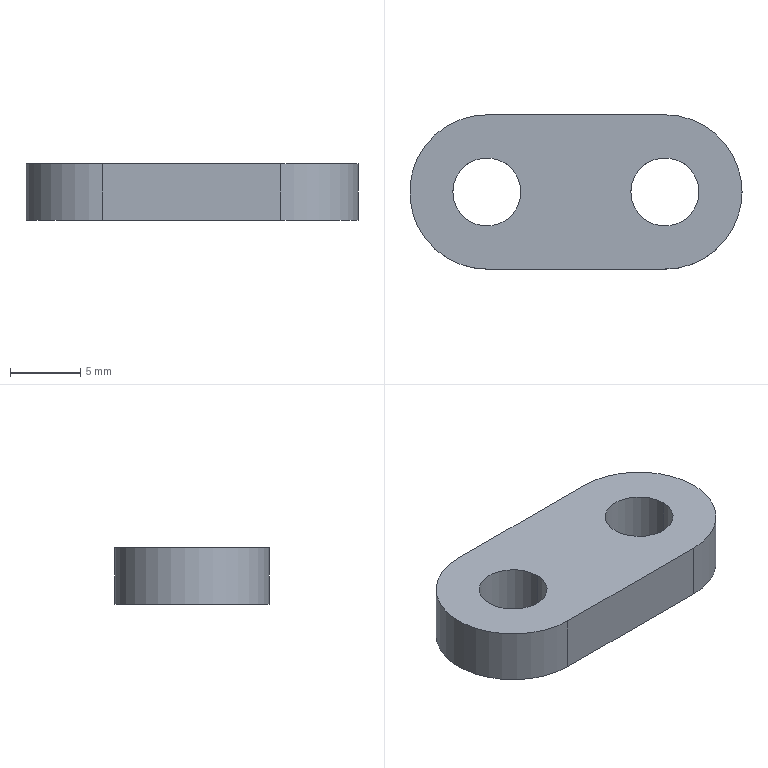Part | STEP file | 11-LINK_MC01-S311 | 1 solid | 11 faces | box 23.697 x 11 x 4 mm | volume 791.004 mm3 | cylinder 7 | plane 4 | commonest cylinder face diameters 4.85 x4 11 x3
STEP:
#1=CARTESIAN_POINT('',(-2.425,0.,-4.));
#2=VERTEX_POINT('',#1);
#3=CARTESIAN_POINT('',(2.425,0.,-4.));
#4=VERTEX_POINT('',#3);
#5=CARTESIAN_POINT('',(0.,0.,-4.));
#6=DIRECTION('',(0.,0.,1.));
#7=DIRECTION('',(1.,0.,0.));
#8=AXIS2_PLACEMENT_3D('',#5,#6,#7);
#9=CIRCLE('',#8,2.425);
#10=EDGE_CURVE('',#2,#4,#9,.T.);
#11=ORIENTED_EDGE('',*,*,#10,.F.);
#12=CARTESIAN_POINT('',(-2.425,0.,0.));
#13=VERTEX_POINT('',#12);
#14=CARTESIAN_POINT('',(-2.425,0.,0.));
#15=DIRECTION('',(0.,0.,1.));
#16=VECTOR('',#15,1000.);
#17=LINE('',#14,#16);
#18=EDGE_CURVE('',#2,#13,#17,.T.);
#19=ORIENTED_EDGE('',*,*,#18,.T.);
#20=CARTESIAN_POINT('',(2.425,0.,0.));
#21=VERTEX_POINT('',#20);
#22=CARTESIAN_POINT('',(0.,0.,0.));
#23=DIRECTION('',(0.,0.,1.));
#24=DIRECTION('',(1.,0.,0.));
#25=AXIS2_PLACEMENT_3D('',#22,#23,#24);
#26=CIRCLE('',#25,2.425);
#27=EDGE_CURVE('',#13,#21,#26,.T.);
#28=ORIENTED_EDGE('',*,*,#27,.T.);
#29=CARTESIAN_POINT('',(2.425,0.,0.));
#30=DIRECTION('',(0.,0.,1.));
#31=VECTOR('',#30,1000.);
#32=LINE('',#29,#31);
#33=EDGE_CURVE('',#4,#21,#32,.T.);
#34=ORIENTED_EDGE('',*,*,#33,.F.);
#35=EDGE_LOOP('',(#11,#19,#28,#34));
#36=FACE_OUTER_BOUND('',#35,.T.);
#37=CARTESIAN_POINT('',(0.,0.,0.));
#38=DIRECTION('',(0.,0.,1.));
#39=DIRECTION('',(1.,0.,0.));
#40=AXIS2_PLACEMENT_3D('',#37,#38,#39);
#41=CYLINDRICAL_SURFACE('',#40,2.425);
#42=ADVANCED_FACE('',(#36),#41,.F.);
#43=CARTESIAN_POINT('',(10.272,0.,-4.));
#44=VERTEX_POINT('',#43);
#45=CARTESIAN_POINT('',(15.122,0.,-4.));
#46=VERTEX_POINT('',#45);
#47=CARTESIAN_POINT('',(12.697,0.,-4.));
#48=DIRECTION('',(0.,0.,1.));
#49=DIRECTION('',(1.,0.,0.));
#50=AXIS2_PLACEMENT_3D('',#47,#48,#49);
#51=CIRCLE('',#50,2.425);
#52=EDGE_CURVE('',#44,#46,#51,.T.);
#53=ORIENTED_EDGE('',*,*,#52,.F.);
#54=CARTESIAN_POINT('',(10.272,0.,0.));
#55=VERTEX_POINT('',#54);
#56=CARTESIAN_POINT('',(10.272,0.,0.));
#57=DIRECTION('',(0.,0.,1.));
#58=VECTOR('',#57,1000.);
#59=LINE('',#56,#58);
#60=EDGE_CURVE('',#44,#55,#59,.T.);
#61=ORIENTED_EDGE('',*,*,#60,.T.);
#62=CARTESIAN_POINT('',(15.122,0.,0.));
#63=VERTEX_POINT('',#62);
#64=CARTESIAN_POINT('',(12.697,0.,0.));
#65=DIRECTION('',(0.,0.,1.));
#66=DIRECTION('',(1.,0.,0.));
#67=AXIS2_PLACEMENT_3D('',#64,#65,#66);
#68=CIRCLE('',#67,2.425);
#69=EDGE_CURVE('',#55,#63,#68,.T.);
#70=ORIENTED_EDGE('',*,*,#69,.T.);
#71=CARTESIAN_POINT('',(15.122,0.,0.));
#72=DIRECTION('',(0.,0.,1.));
#73=VECTOR('',#72,1000.);
#74=LINE('',#71,#73);
#75=EDGE_CURVE('',#46,#63,#74,.T.);
#76=ORIENTED_EDGE('',*,*,#75,.F.);
#77=EDGE_LOOP('',(#53,#61,#70,#76));
#78=FACE_OUTER_BOUND('',#77,.T.);
#79=CARTESIAN_POINT('',(12.697,0.,0.));
#80=DIRECTION('',(0.,0.,1.));
#81=DIRECTION('',(1.,0.,0.));
#82=AXIS2_PLACEMENT_3D('',#79,#80,#81);
#83=CYLINDRICAL_SURFACE('',#82,2.425);
#84=ADVANCED_FACE('',(#78),#83,.F.);
#85=CARTESIAN_POINT('',(12.697,-5.5,-4.));
#86=VERTEX_POINT('',#85);
#87=CARTESIAN_POINT('',(18.197,0.,-4.));
#88=VERTEX_POINT('',#87);
#89=CARTESIAN_POINT('',(12.697,0.,-4.));
#90=DIRECTION('',(0.,0.,1.));
#91=DIRECTION('',(1.,0.,0.));
#92=AXIS2_PLACEMENT_3D('',#89,#90,#91);
#93=CIRCLE('',#92,5.5);
#94=EDGE_CURVE('',#86,#88,#93,.T.);
#95=ORIENTED_EDGE('',*,*,#94,.T.);
#96=CARTESIAN_POINT('',(18.197,0.,0.));
#97=VERTEX_POINT('',#96);
#98=CARTESIAN_POINT('',(18.197,0.,-4.));
#99=DIRECTION('',(0.,0.,1.));
#100=VECTOR('',#99,1000.);
#101=LINE('',#98,#100);
#102=EDGE_CURVE('',#88,#97,#101,.T.);
#103=ORIENTED_EDGE('',*,*,#102,.T.);
#104=CARTESIAN_POINT('',(12.697,-5.5,0.));
#105=VERTEX_POINT('',#104);
#106=CARTESIAN_POINT('',(12.697,0.,0.));
#107=DIRECTION('',(0.,0.,1.));
#108=DIRECTION('',(1.,0.,0.));
#109=AXIS2_PLACEMENT_3D('',#106,#107,#108);
#110=CIRCLE('',#109,5.5);
#111=EDGE_CURVE('',#105,#97,#110,.T.);
#112=ORIENTED_EDGE('',*,*,#111,.F.);
#113=CARTESIAN_POINT('',(12.697,-5.5,-4.));
#114=DIRECTION('',(0.,0.,1.));
#115=VECTOR('',#114,1000.);
#116=LINE('',#113,#115);
#117=EDGE_CURVE('',#86,#105,#116,.T.);
#118=ORIENTED_EDGE('',*,*,#117,.F.);
#119=EDGE_LOOP('',(#95,#103,#112,#118));
#120=FACE_OUTER_BOUND('',#119,.T.);
#121=CARTESIAN_POINT('',(12.697,0.,-4.));
#122=DIRECTION('',(0.,0.,1.));
#123=DIRECTION('',(1.,0.,0.));
#124=AXIS2_PLACEMENT_3D('',#121,#122,#123);
#125=CYLINDRICAL_SURFACE('',#124,5.5);
#126=ADVANCED_FACE('',(#120),#125,.T.);
#127=CARTESIAN_POINT('',(0.,5.5,0.));
#128=VERTEX_POINT('',#127);
#129=CARTESIAN_POINT('',(0.,-5.5,0.));
#130=VERTEX_POINT('',#129);
#131=CARTESIAN_POINT('',(0.,0.,0.));
#132=DIRECTION('',(0.,0.,1.));
#133=DIRECTION('',(1.,0.,0.));
#134=AXIS2_PLACEMENT_3D('',#131,#132,#133);
#135=CIRCLE('',#134,5.5);
#136=EDGE_CURVE('',#128,#130,#135,.T.);
#137=ORIENTED_EDGE('',*,*,#136,.F.);
#138=CARTESIAN_POINT('',(0.,5.5,-4.));
#139=VERTEX_POINT('',#138);
#140=CARTESIAN_POINT('',(0.,5.5,-4.));
#141=DIRECTION('',(0.,0.,1.));
#142=VECTOR('',#141,1000.);
#143=LINE('',#140,#142);
#144=EDGE_CURVE('',#139,#128,#143,.T.);
#145=ORIENTED_EDGE('',*,*,#144,.F.);
#146=CARTESIAN_POINT('',(0.,-5.5,-4.));
#147=VERTEX_POINT('',#146);
#148=CARTESIAN_POINT('',(0.,0.,-4.));
#149=DIRECTION('',(0.,0.,1.));
#150=DIRECTION('',(1.,0.,0.));
#151=AXIS2_PLACEMENT_3D('',#148,#149,#150);
#152=CIRCLE('',#151,5.5);
#153=EDGE_CURVE('',#139,#147,#152,.T.);
#154=ORIENTED_EDGE('',*,*,#153,.T.);
#155=CARTESIAN_POINT('',(0.,-5.5,-4.));
#156=DIRECTION('',(0.,0.,1.));
#157=VECTOR('',#156,1000.);
#158=LINE('',#155,#157);
#159=EDGE_CURVE('',#147,#130,#158,.T.);
#160=ORIENTED_EDGE('',*,*,#159,.T.);
#161=EDGE_LOOP('',(#137,#145,#154,#160));
#162=FACE_OUTER_BOUND('',#161,.T.);
#163=CARTESIAN_POINT('',(0.,0.,-4.));
#164=DIRECTION('',(0.,0.,1.));
#165=DIRECTION('',(1.,0.,0.));
#166=AXIS2_PLACEMENT_3D('',#163,#164,#165);
#167=CYLINDRICAL_SURFACE('',#166,5.5);
#168=ADVANCED_FACE('',(#162),#167,.T.);
#169=CARTESIAN_POINT('',(12.697,5.5,0.));
#170=VERTEX_POINT('',#169);
#171=CARTESIAN_POINT('',(0.,5.5,0.));
#172=DIRECTION('',(-1.,0.,0.));
#173=VECTOR('',#172,1000.);
#174=LINE('',#171,#173);
#175=EDGE_CURVE('',#170,#128,#174,.T.);
#176=ORIENTED_EDGE('',*,*,#175,.F.);
#177=CARTESIAN_POINT('',(12.697,5.5,-4.));
#178=VERTEX_POINT('',#177);
#179=CARTESIAN_POINT('',(12.697,5.5,-4.));
#180=DIRECTION('',(0.,0.,1.));
#181=VECTOR('',#180,1000.);
#182=LINE('',#179,#181);
#183=EDGE_CURVE('',#178,#170,#182,.T.);
#184=ORIENTED_EDGE('',*,*,#183,.F.);
#185=CARTESIAN_POINT('',(0.,5.5,-4.));
#186=DIRECTION('',(-1.,0.,0.));
#187=VECTOR('',#186,1000.);
#188=LINE('',#185,#187);
#189=EDGE_CURVE('',#178,#139,#188,.T.);
#190=ORIENTED_EDGE('',*,*,#189,.T.);
#191=ORIENTED_EDGE('',*,*,#144,.T.);
#192=EDGE_LOOP('',(#176,#184,#190,#191));
#193=FACE_OUTER_BOUND('',#192,.T.);
#194=CARTESIAN_POINT('',(0.,5.5,-4.));
#195=DIRECTION('',(0.,1.,0.));
#196=DIRECTION('',(0.,0.,1.));
#197=AXIS2_PLACEMENT_3D('',#194,#195,#196);
#198=PLANE('',#197);
#199=ADVANCED_FACE('',(#193),#198,.T.);
#200=ORIENTED_EDGE('',*,*,#102,.F.);
#201=CARTESIAN_POINT('',(12.697,0.,-4.));
#202=DIRECTION('',(0.,0.,1.));
#203=DIRECTION('',(1.,0.,0.));
#204=AXIS2_PLACEMENT_3D('',#201,#202,#203);
#205=CIRCLE('',#204,5.5);
#206=EDGE_CURVE('',#88,#178,#205,.T.);
#207=ORIENTED_EDGE('',*,*,#206,.T.);
#208=ORIENTED_EDGE('',*,*,#183,.T.);
#209=CARTESIAN_POINT('',(12.697,0.,0.));
#210=DIRECTION('',(0.,0.,1.));
#211=DIRECTION('',(1.,0.,0.));
#212=AXIS2_PLACEMENT_3D('',#209,#210,#211);
#213=CIRCLE('',#212,5.5);
#214=EDGE_CURVE('',#97,#170,#213,.T.);
#215=ORIENTED_EDGE('',*,*,#214,.F.);
#216=EDGE_LOOP('',(#200,#207,#208,#215));
#217=FACE_OUTER_BOUND('',#216,.T.);
#218=CARTESIAN_POINT('',(12.697,0.,-4.));
#219=DIRECTION('',(0.,0.,1.));
#220=DIRECTION('',(1.,0.,0.));
#221=AXIS2_PLACEMENT_3D('',#218,#219,#220);
#222=CYLINDRICAL_SURFACE('',#221,5.5);
#223=ADVANCED_FACE('',(#217),#222,.T.);
#224=CARTESIAN_POINT('',(0.,-5.5,0.));
#225=DIRECTION('',(1.,0.,0.));
#226=VECTOR('',#225,1000.);
#227=LINE('',#224,#226);
#228=EDGE_CURVE('',#130,#105,#227,.T.);
#229=ORIENTED_EDGE('',*,*,#228,.F.);
#230=ORIENTED_EDGE('',*,*,#159,.F.);
#231=CARTESIAN_POINT('',(0.,-5.5,-4.));
#232=DIRECTION('',(1.,0.,0.));
#233=VECTOR('',#232,1000.);
#234=LINE('',#231,#233);
#235=EDGE_CURVE('',#147,#86,#234,.T.);
#236=ORIENTED_EDGE('',*,*,#235,.T.);
#237=ORIENTED_EDGE('',*,*,#117,.T.);
#238=EDGE_LOOP('',(#229,#230,#236,#237));
#239=FACE_OUTER_BOUND('',#238,.T.);
#240=CARTESIAN_POINT('',(0.,-5.5,-4.));
#241=DIRECTION('',(0.,-1.,0.));
#242=DIRECTION('',(0.,0.,-1.));
#243=AXIS2_PLACEMENT_3D('',#240,#241,#242);
#244=PLANE('',#243);
#245=ADVANCED_FACE('',(#239),#244,.T.);
#246=CARTESIAN_POINT('',(0.,0.,-4.));
#247=DIRECTION('',(0.,0.,1.));
#248=DIRECTION('',(1.,0.,0.));
#249=AXIS2_PLACEMENT_3D('',#246,#247,#248);
#250=CIRCLE('',#249,2.425);
#251=EDGE_CURVE('',#4,#2,#250,.T.);
#252=ORIENTED_EDGE('',*,*,#251,.T.);
#253=ORIENTED_EDGE('',*,*,#10,.T.);
#254=EDGE_LOOP('',(#252,#253));
#255=FACE_BOUND('',#254,.T.);
#256=CARTESIAN_POINT('',(12.697,0.,-4.));
#257=DIRECTION('',(0.,0.,1.));
#258=DIRECTION('',(1.,0.,0.));
#259=AXIS2_PLACEMENT_3D('',#256,#257,#258);
#260=CIRCLE('',#259,2.425);
#261=EDGE_CURVE('',#46,#44,#260,.T.);
#262=ORIENTED_EDGE('',*,*,#261,.T.);
#263=ORIENTED_EDGE('',*,*,#52,.T.);
#264=EDGE_LOOP('',(#262,#263));
#265=FACE_BOUND('',#264,.T.);
#266=ORIENTED_EDGE('',*,*,#153,.F.);
#267=ORIENTED_EDGE('',*,*,#189,.F.);
#268=ORIENTED_EDGE('',*,*,#206,.F.);
#269=ORIENTED_EDGE('',*,*,#94,.F.);
#270=ORIENTED_EDGE('',*,*,#235,.F.);
#271=EDGE_LOOP('',(#266,#267,#268,#269,#270));
#272=FACE_OUTER_BOUND('',#271,.T.);
#273=CARTESIAN_POINT('',(0.,0.,-4.));
#274=DIRECTION('',(0.,0.,1.));
#275=DIRECTION('',(1.,0.,0.));
#276=AXIS2_PLACEMENT_3D('',#273,#274,#275);
#277=PLANE('',#276);
#278=ADVANCED_FACE('',(#255,#265,#272),#277,.F.);
#279=CARTESIAN_POINT('',(0.,0.,0.));
#280=DIRECTION('',(0.,0.,1.));
#281=DIRECTION('',(1.,0.,0.));
#282=AXIS2_PLACEMENT_3D('',#279,#280,#281);
#283=CIRCLE('',#282,2.425);
#284=EDGE_CURVE('',#21,#13,#283,.T.);
#285=ORIENTED_EDGE('',*,*,#284,.F.);
#286=ORIENTED_EDGE('',*,*,#27,.F.);
#287=EDGE_LOOP('',(#285,#286));
#288=FACE_BOUND('',#287,.T.);
#289=CARTESIAN_POINT('',(12.697,0.,0.));
#290=DIRECTION('',(0.,0.,1.));
#291=DIRECTION('',(1.,0.,0.));
#292=AXIS2_PLACEMENT_3D('',#289,#290,#291);
#293=CIRCLE('',#292,2.425);
#294=EDGE_CURVE('',#63,#55,#293,.T.);
#295=ORIENTED_EDGE('',*,*,#294,.F.);
#296=ORIENTED_EDGE('',*,*,#69,.F.);
#297=EDGE_LOOP('',(#295,#296));
#298=FACE_BOUND('',#297,.T.);
#299=ORIENTED_EDGE('',*,*,#136,.T.);
#300=ORIENTED_EDGE('',*,*,#228,.T.);
#301=ORIENTED_EDGE('',*,*,#111,.T.);
#302=ORIENTED_EDGE('',*,*,#214,.T.);
#303=ORIENTED_EDGE('',*,*,#175,.T.);
#304=EDGE_LOOP('',(#299,#300,#301,#302,#303));
#305=FACE_OUTER_BOUND('',#304,.T.);
#306=CARTESIAN_POINT('',(0.,0.,0.));
#307=DIRECTION('',(0.,0.,1.));
#308=DIRECTION('',(1.,0.,0.));
#309=AXIS2_PLACEMENT_3D('',#306,#307,#308);
#310=PLANE('',#309);
#311=ADVANCED_FACE('',(#288,#298,#305),#310,.T.);
#312=ORIENTED_EDGE('',*,*,#60,.F.);
#313=ORIENTED_EDGE('',*,*,#261,.F.);
#314=ORIENTED_EDGE('',*,*,#75,.T.);
#315=ORIENTED_EDGE('',*,*,#294,.T.);
#316=EDGE_LOOP('',(#312,#313,#314,#315));
#317=FACE_OUTER_BOUND('',#316,.T.);
#318=CARTESIAN_POINT('',(12.697,0.,0.));
#319=DIRECTION('',(0.,0.,1.));
#320=DIRECTION('',(1.,0.,0.));
#321=AXIS2_PLACEMENT_3D('',#318,#319,#320);
#322=CYLINDRICAL_SURFACE('',#321,2.425);
#323=ADVANCED_FACE('',(#317),#322,.F.);
#324=ORIENTED_EDGE('',*,*,#18,.F.);
#325=ORIENTED_EDGE('',*,*,#251,.F.);
#326=ORIENTED_EDGE('',*,*,#33,.T.);
#327=ORIENTED_EDGE('',*,*,#284,.T.);
#328=EDGE_LOOP('',(#324,#325,#326,#327));
#329=FACE_OUTER_BOUND('',#328,.T.);
#330=CARTESIAN_POINT('',(0.,0.,0.));
#331=DIRECTION('',(0.,0.,1.));
#332=DIRECTION('',(1.,0.,0.));
#333=AXIS2_PLACEMENT_3D('',#330,#331,#332);
#334=CYLINDRICAL_SURFACE('',#333,2.425);
#335=ADVANCED_FACE('',(#329),#334,.F.);
#336=CLOSED_SHELL('',(#42,#84,#126,#168,#199,#223,#245,#278,#311,#323,#335));
#337=MANIFOLD_SOLID_BREP('',#336);
#338=CARTESIAN_POINT('',(0.,0.,0.));
#339=DIRECTION('',(0.,0.,1.));
#340=DIRECTION('',(1.,0.,0.));
#341=AXIS2_PLACEMENT_3D('',#338,#339,#340);
#342=(LENGTH_UNIT()NAMED_UNIT(*)SI_UNIT(.MILLI.,.METRE.));
#343=UNCERTAINTY_MEASURE_WITH_UNIT(LENGTH_MEASURE(0.00001),#342,'','');
#344=(NAMED_UNIT(*)PLANE_ANGLE_UNIT()SI_UNIT($,.RADIAN.));
#345=(NAMED_UNIT(*)SI_UNIT($,.STERADIAN.)SOLID_ANGLE_UNIT());
#346=(GEOMETRIC_REPRESENTATION_CONTEXT(3)GLOBAL_UNCERTAINTY_ASSIGNED_CONTEXT((#343))GLOBAL_UNIT_ASSIGNED_CONTEXT((#342,#344,#345))REPRESENTATION_CONTEXT('',''));
#347=ADVANCED_BREP_SHAPE_REPRESENTATION('',(#337,#341),#346);